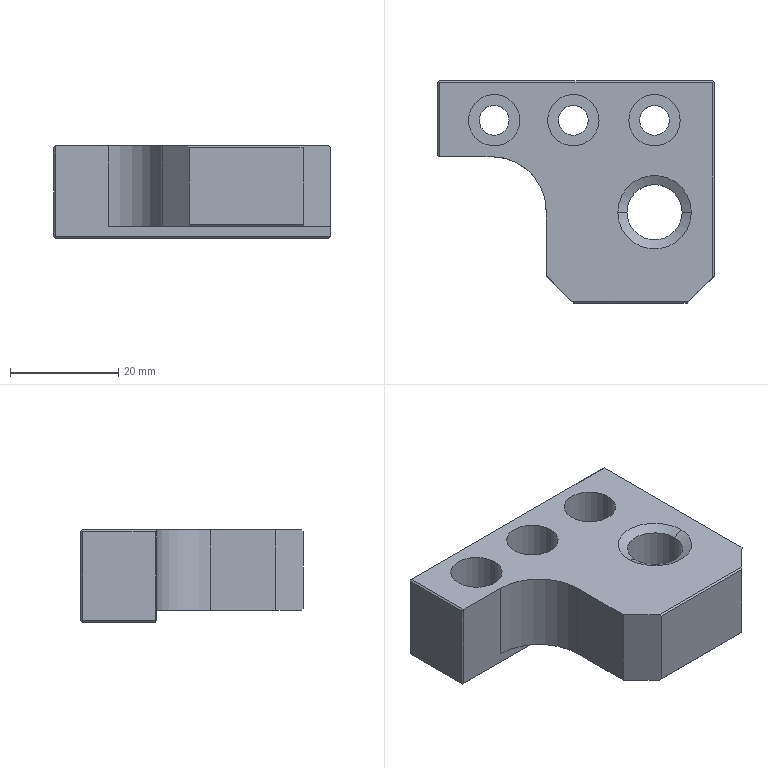Part | NX | 1 solid | 43 faces | box 51 x 41 x 17 mm | volume 20948 mm3 | plane 26 | cylinder 15 | cone 2 | commonest cylinder face diameters 5.5 x6 9.5 x6 10.2 x2 20 x1
STEP:
#1=CARTESIAN_POINT('',(1547.5,164.7,-33.6));
#2=VERTEX_POINT('',#1);
#3=CARTESIAN_POINT('',(1547.5,151.,-33.6));
#4=VERTEX_POINT('',#3);
#5=CARTESIAN_POINT('',(1547.5,165.,-33.6));
#6=DIRECTION('',(0.,-1.,0.));
#7=VECTOR('',#6,1000.);
#8=LINE('',#5,#7);
#9=EDGE_CURVE('',#2,#4,#8,.T.);
#10=ORIENTED_EDGE('',*,*,#9,.F.);
#11=CARTESIAN_POINT('',(1547.5,164.7,-17.2));
#12=VERTEX_POINT('',#11);
#13=CARTESIAN_POINT('',(1547.5,164.7,-25.4));
#14=DIRECTION('',(0.,0.,-1.));
#15=VECTOR('',#14,1000.);
#16=LINE('',#13,#15);
#17=EDGE_CURVE('',#12,#2,#16,.T.);
#18=ORIENTED_EDGE('',*,*,#17,.F.);
#19=CARTESIAN_POINT('',(1547.5,129.,-17.2));
#20=VERTEX_POINT('',#19);
#21=CARTESIAN_POINT('',(1547.5,147.,-17.2));
#22=DIRECTION('',(0.,-1.,0.));
#23=VECTOR('',#22,1000.);
#24=LINE('',#21,#23);
#25=EDGE_CURVE('',#12,#20,#24,.T.);
#26=ORIENTED_EDGE('',*,*,#25,.T.);
#27=CARTESIAN_POINT('',(1547.5,129.,-31.7));
#28=VERTEX_POINT('',#27);
#29=CARTESIAN_POINT('',(1547.5,129.,-24.3));
#30=DIRECTION('',(0.,0.,1.));
#31=VECTOR('',#30,1000.);
#32=LINE('',#29,#31);
#33=EDGE_CURVE('',#28,#20,#32,.T.);
#34=ORIENTED_EDGE('',*,*,#33,.F.);
#35=CARTESIAN_POINT('',(1547.5,151.,-31.7));
#36=VERTEX_POINT('',#35);
#37=CARTESIAN_POINT('',(1547.5,165.,-31.7));
#38=DIRECTION('',(0.,-1.,0.));
#39=VECTOR('',#38,1000.);
#40=LINE('',#37,#39);
#41=EDGE_CURVE('',#36,#28,#40,.T.);
#42=ORIENTED_EDGE('',*,*,#41,.F.);
#43=CARTESIAN_POINT('',(1547.5,151.,-40.046));
#44=DIRECTION('',(0.,0.,1.));
#45=VECTOR('',#44,1000.);
#46=LINE('',#43,#45);
#47=EDGE_CURVE('',#4,#36,#46,.T.);
#48=ORIENTED_EDGE('',*,*,#47,.F.);
#49=EDGE_LOOP('',(#10,#18,#26,#34,#42,#48));
#50=FACE_BOUND('',#49,.T.);
#51=CARTESIAN_POINT('',(1547.5,165.,-12.9));
#52=DIRECTION('',(1.,0.,0.));
#53=DIRECTION('',(0.,1.,0.));
#54=AXIS2_PLACEMENT_3D('',#51,#52,#53);
#55=PLANE('',#54);
#56=ADVANCED_FACE('',(#50),#55,.T.);
#57=CARTESIAN_POINT('',(1496.8,151.,-16.9));
#58=VERTEX_POINT('',#57);
#59=CARTESIAN_POINT('',(1496.8,164.7,-16.9));
#60=VERTEX_POINT('',#59);
#61=CARTESIAN_POINT('',(1496.8,165.,-16.9));
#62=DIRECTION('',(0.,1.,0.));
#63=VECTOR('',#62,1000.);
#64=LINE('',#61,#63);
#65=EDGE_CURVE('',#58,#60,#64,.T.);
#66=ORIENTED_EDGE('',*,*,#65,.F.);
#67=CARTESIAN_POINT('',(1506.5,151.,-16.9));
#68=VERTEX_POINT('',#67);
#69=CARTESIAN_POINT('',(1509.731,151.,-16.9));
#70=DIRECTION('',(-1.,0.,0.));
#71=VECTOR('',#70,1000.);
#72=LINE('',#69,#71);
#73=EDGE_CURVE('',#68,#58,#72,.T.);
#74=ORIENTED_EDGE('',*,*,#73,.F.);
#75=CARTESIAN_POINT('',(1516.5,141.,-16.9));
#76=VERTEX_POINT('',#75);
#77=CARTESIAN_POINT('',(1506.5,141.,-16.9));
#78=DIRECTION('',(0.,0.,1.));
#79=DIRECTION('',(0.,-1.,0.));
#80=AXIS2_PLACEMENT_3D('',#77,#78,#79);
#81=CIRCLE('',#80,10.);
#82=EDGE_CURVE('',#76,#68,#81,.T.);
#83=ORIENTED_EDGE('',*,*,#82,.F.);
#84=CARTESIAN_POINT('',(1516.5,129.,-16.9));
#85=VERTEX_POINT('',#84);
#86=CARTESIAN_POINT('',(1516.5,165.,-16.9));
#87=DIRECTION('',(0.,1.,0.));
#88=VECTOR('',#87,1000.);
#89=LINE('',#86,#88);
#90=EDGE_CURVE('',#85,#76,#89,.T.);
#91=ORIENTED_EDGE('',*,*,#90,.F.);
#92=CARTESIAN_POINT('',(1521.2,124.3,-16.9));
#93=VERTEX_POINT('',#92);
#94=CARTESIAN_POINT('',(1480.5,165.,-16.9));
#95=DIRECTION('',(0.7071,-0.7071,0.));
#96=VECTOR('',#95,1000.);
#97=LINE('',#94,#96);
#98=EDGE_CURVE('',#85,#93,#97,.T.);
#99=ORIENTED_EDGE('',*,*,#98,.T.);
#100=CARTESIAN_POINT('',(1542.8,124.3,-16.9));
#101=VERTEX_POINT('',#100);
#102=CARTESIAN_POINT('',(1532.,124.3,-16.9));
#103=DIRECTION('',(-1.,0.,0.));
#104=VECTOR('',#103,1000.);
#105=LINE('',#102,#104);
#106=EDGE_CURVE('',#101,#93,#105,.T.);
#107=ORIENTED_EDGE('',*,*,#106,.F.);
#108=CARTESIAN_POINT('',(1547.2,128.7,-16.9));
#109=VERTEX_POINT('',#108);
#110=CARTESIAN_POINT('',(1583.5,165.,-16.9));
#111=DIRECTION('',(-0.7071,-0.7071,0.));
#112=VECTOR('',#111,1000.);
#113=LINE('',#110,#112);
#114=EDGE_CURVE('',#109,#101,#113,.T.);
#115=ORIENTED_EDGE('',*,*,#114,.F.);
#116=CARTESIAN_POINT('',(1547.2,164.7,-16.9));
#117=VERTEX_POINT('',#116);
#118=CARTESIAN_POINT('',(1547.2,147.,-16.9));
#119=DIRECTION('',(0.,-1.,0.));
#120=VECTOR('',#119,1000.);
#121=LINE('',#118,#120);
#122=EDGE_CURVE('',#117,#109,#121,.T.);
#123=ORIENTED_EDGE('',*,*,#122,.F.);
#124=CARTESIAN_POINT('',(1522.,164.7,-16.9));
#125=DIRECTION('',(1.,0.,0.));
#126=VECTOR('',#125,1000.);
#127=LINE('',#124,#126);
#128=EDGE_CURVE('',#60,#117,#127,.T.);
#129=ORIENTED_EDGE('',*,*,#128,.F.);
#130=EDGE_LOOP('',(#66,#74,#83,#91,#99,#107,#115,#123,#129));
#131=FACE_BOUND('',#130,.T.);
#132=CARTESIAN_POINT('',(1543.287,140.75,-16.9));
#133=VERTEX_POINT('',#132);
#134=CARTESIAN_POINT('',(1529.713,140.75,-16.9));
#135=VERTEX_POINT('',#134);
#136=CARTESIAN_POINT('',(1536.5,140.75,-16.9));
#137=DIRECTION('',(0.,0.,1.));
#138=DIRECTION('',(-1.,0.,0.));
#139=AXIS2_PLACEMENT_3D('',#136,#137,#138);
#140=CIRCLE('',#139,6.787);
#141=EDGE_CURVE('',#133,#135,#140,.T.);
#142=ORIENTED_EDGE('',*,*,#141,.F.);
#143=CARTESIAN_POINT('',(1536.5,140.75,-16.9));
#144=DIRECTION('',(0.,0.,1.));
#145=DIRECTION('',(-1.,0.,0.));
#146=AXIS2_PLACEMENT_3D('',#143,#144,#145);
#147=CIRCLE('',#146,6.787);
#148=EDGE_CURVE('',#135,#133,#147,.T.);
#149=ORIENTED_EDGE('',*,*,#148,.F.);
#150=EDGE_LOOP('',(#142,#149));
#151=FACE_BOUND('',#150,.T.);
#152=CARTESIAN_POINT('',(1541.25,157.75,-16.9));
#153=VERTEX_POINT('',#152);
#154=CARTESIAN_POINT('',(1531.75,157.75,-16.9));
#155=VERTEX_POINT('',#154);
#156=CARTESIAN_POINT('',(1536.5,157.75,-16.9));
#157=DIRECTION('',(0.,0.,1.));
#158=DIRECTION('',(-1.,0.,0.));
#159=AXIS2_PLACEMENT_3D('',#156,#157,#158);
#160=CIRCLE('',#159,4.75);
#161=EDGE_CURVE('',#153,#155,#160,.T.);
#162=ORIENTED_EDGE('',*,*,#161,.F.);
#163=CARTESIAN_POINT('',(1536.5,157.75,-16.9));
#164=DIRECTION('',(0.,0.,1.));
#165=DIRECTION('',(-1.,0.,0.));
#166=AXIS2_PLACEMENT_3D('',#163,#164,#165);
#167=CIRCLE('',#166,4.75);
#168=EDGE_CURVE('',#155,#153,#167,.T.);
#169=ORIENTED_EDGE('',*,*,#168,.F.);
#170=EDGE_LOOP('',(#162,#169));
#171=FACE_BOUND('',#170,.T.);
#172=CARTESIAN_POINT('',(1511.642,157.75,-16.9));
#173=VERTEX_POINT('',#172);
#174=CARTESIAN_POINT('',(1502.142,157.75,-16.9));
#175=VERTEX_POINT('',#174);
#176=CARTESIAN_POINT('',(1506.892,157.75,-16.9));
#177=DIRECTION('',(0.,0.,1.));
#178=DIRECTION('',(-1.,0.,0.));
#179=AXIS2_PLACEMENT_3D('',#176,#177,#178);
#180=CIRCLE('',#179,4.75);
#181=EDGE_CURVE('',#173,#175,#180,.T.);
#182=ORIENTED_EDGE('',*,*,#181,.F.);
#183=CARTESIAN_POINT('',(1506.892,157.75,-16.9));
#184=DIRECTION('',(0.,0.,1.));
#185=DIRECTION('',(-1.,0.,0.));
#186=AXIS2_PLACEMENT_3D('',#183,#184,#185);
#187=CIRCLE('',#186,4.75);
#188=EDGE_CURVE('',#175,#173,#187,.T.);
#189=ORIENTED_EDGE('',*,*,#188,.F.);
#190=EDGE_LOOP('',(#182,#189));
#191=FACE_BOUND('',#190,.T.);
#192=CARTESIAN_POINT('',(1526.25,157.75,-16.9));
#193=VERTEX_POINT('',#192);
#194=CARTESIAN_POINT('',(1516.75,157.75,-16.9));
#195=VERTEX_POINT('',#194);
#196=CARTESIAN_POINT('',(1521.5,157.75,-16.9));
#197=DIRECTION('',(0.,0.,1.));
#198=DIRECTION('',(-1.,0.,0.));
#199=AXIS2_PLACEMENT_3D('',#196,#197,#198);
#200=CIRCLE('',#199,4.75);
#201=EDGE_CURVE('',#193,#195,#200,.T.);
#202=ORIENTED_EDGE('',*,*,#201,.F.);
#203=CARTESIAN_POINT('',(1521.5,157.75,-16.9));
#204=DIRECTION('',(0.,0.,1.));
#205=DIRECTION('',(-1.,0.,0.));
#206=AXIS2_PLACEMENT_3D('',#203,#204,#205);
#207=CIRCLE('',#206,4.75);
#208=EDGE_CURVE('',#195,#193,#207,.T.);
#209=ORIENTED_EDGE('',*,*,#208,.F.);
#210=EDGE_LOOP('',(#202,#209));
#211=FACE_BOUND('',#210,.T.);
#212=CARTESIAN_POINT('',(1491.5,165.,-16.9));
#213=DIRECTION('',(0.,0.,1.));
#214=DIRECTION('',(0.,-1.,0.));
#215=AXIS2_PLACEMENT_3D('',#212,#213,#214);
#216=PLANE('',#215);
#217=ADVANCED_FACE('',(#131,#151,#171,#191,#211),#216,.T.);
#218=CARTESIAN_POINT('',(1496.5,151.3,-17.2));
#219=VERTEX_POINT('',#218);
#220=CARTESIAN_POINT('',(1496.5,151.3,-33.6));
#221=VERTEX_POINT('',#220);
#222=CARTESIAN_POINT('',(1496.5,151.3,-25.4));
#223=DIRECTION('',(0.,0.,-1.));
#224=VECTOR('',#223,1000.);
#225=LINE('',#222,#224);
#226=EDGE_CURVE('',#219,#221,#225,.T.);
#227=ORIENTED_EDGE('',*,*,#226,.F.);
#228=CARTESIAN_POINT('',(1496.5,164.7,-17.2));
#229=VERTEX_POINT('',#228);
#230=CARTESIAN_POINT('',(1496.5,165.,-17.2));
#231=DIRECTION('',(0.,1.,0.));
#232=VECTOR('',#231,1000.);
#233=LINE('',#230,#232);
#234=EDGE_CURVE('',#219,#229,#233,.T.);
#235=ORIENTED_EDGE('',*,*,#234,.T.);
#236=CARTESIAN_POINT('',(1496.5,164.7,-33.6));
#237=VERTEX_POINT('',#236);
#238=CARTESIAN_POINT('',(1496.5,164.7,-25.4));
#239=DIRECTION('',(0.,0.,1.));
#240=VECTOR('',#239,1000.);
#241=LINE('',#238,#240);
#242=EDGE_CURVE('',#237,#229,#241,.T.);
#243=ORIENTED_EDGE('',*,*,#242,.F.);
#244=CARTESIAN_POINT('',(1496.5,165.,-33.6));
#245=DIRECTION('',(0.,1.,0.));
#246=VECTOR('',#245,1000.);
#247=LINE('',#244,#246);
#248=EDGE_CURVE('',#221,#237,#247,.T.);
#249=ORIENTED_EDGE('',*,*,#248,.F.);
#250=EDGE_LOOP('',(#227,#235,#243,#249));
#251=FACE_BOUND('',#250,.T.);
#252=CARTESIAN_POINT('',(1496.5,165.,-33.9));
#253=DIRECTION('',(-1.,0.,0.));
#254=DIRECTION('',(0.,0.,1.));
#255=AXIS2_PLACEMENT_3D('',#252,#253,#254);
#256=PLANE('',#255);
#257=ADVANCED_FACE('',(#251),#256,.T.);
#258=CARTESIAN_POINT('',(1496.8,151.3,-33.9));
#259=VERTEX_POINT('',#258);
#260=CARTESIAN_POINT('',(1496.8,164.7,-33.9));
#261=VERTEX_POINT('',#260);
#262=CARTESIAN_POINT('',(1496.8,165.,-33.9));
#263=DIRECTION('',(0.,1.,0.));
#264=VECTOR('',#263,1000.);
#265=LINE('',#262,#264);
#266=EDGE_CURVE('',#259,#261,#265,.T.);
#267=ORIENTED_EDGE('',*,*,#266,.T.);
#268=CARTESIAN_POINT('',(1547.2,164.7,-33.9));
#269=VERTEX_POINT('',#268);
#270=CARTESIAN_POINT('',(1522.,164.7,-33.9));
#271=DIRECTION('',(1.,0.,0.));
#272=VECTOR('',#271,1000.);
#273=LINE('',#270,#272);
#274=EDGE_CURVE('',#261,#269,#273,.T.);
#275=ORIENTED_EDGE('',*,*,#274,.T.);
#276=CARTESIAN_POINT('',(1547.2,151.3,-33.9));
#277=VERTEX_POINT('',#276);
#278=CARTESIAN_POINT('',(1547.2,165.,-33.9));
#279=DIRECTION('',(0.,-1.,0.));
#280=VECTOR('',#279,1000.);
#281=LINE('',#278,#280);
#282=EDGE_CURVE('',#269,#277,#281,.T.);
#283=ORIENTED_EDGE('',*,*,#282,.T.);
#284=CARTESIAN_POINT('',(1522.,151.3,-33.9));
#285=DIRECTION('',(1.,0.,0.));
#286=VECTOR('',#285,1000.);
#287=LINE('',#284,#286);
#288=EDGE_CURVE('',#259,#277,#287,.T.);
#289=ORIENTED_EDGE('',*,*,#288,.F.);
#290=EDGE_LOOP('',(#267,#275,#283,#289));
#291=FACE_BOUND('',#290,.T.);
#292=CARTESIAN_POINT('',(1509.642,157.75,-33.9));
#293=VERTEX_POINT('',#292);
#294=CARTESIAN_POINT('',(1504.142,157.75,-33.9));
#295=VERTEX_POINT('',#294);
#296=CARTESIAN_POINT('',(1506.892,157.75,-33.9));
#297=DIRECTION('',(0.,0.,1.));
#298=DIRECTION('',(-1.,0.,0.));
#299=AXIS2_PLACEMENT_3D('',#296,#297,#298);
#300=CIRCLE('',#299,2.75);
#301=EDGE_CURVE('',#293,#295,#300,.T.);
#302=ORIENTED_EDGE('',*,*,#301,.T.);
#303=CARTESIAN_POINT('',(1506.892,157.75,-33.9));
#304=DIRECTION('',(0.,0.,1.));
#305=DIRECTION('',(-1.,0.,0.));
#306=AXIS2_PLACEMENT_3D('',#303,#304,#305);
#307=CIRCLE('',#306,2.75);
#308=EDGE_CURVE('',#295,#293,#307,.T.);
#309=ORIENTED_EDGE('',*,*,#308,.T.);
#310=EDGE_LOOP('',(#302,#309));
#311=FACE_BOUND('',#310,.T.);
#312=CARTESIAN_POINT('',(1524.25,157.75,-33.9));
#313=VERTEX_POINT('',#312);
#314=CARTESIAN_POINT('',(1518.75,157.75,-33.9));
#315=VERTEX_POINT('',#314);
#316=CARTESIAN_POINT('',(1521.5,157.75,-33.9));
#317=DIRECTION('',(0.,0.,1.));
#318=DIRECTION('',(-1.,0.,0.));
#319=AXIS2_PLACEMENT_3D('',#316,#317,#318);
#320=CIRCLE('',#319,2.75);
#321=EDGE_CURVE('',#313,#315,#320,.T.);
#322=ORIENTED_EDGE('',*,*,#321,.T.);
#323=CARTESIAN_POINT('',(1521.5,157.75,-33.9));
#324=DIRECTION('',(0.,0.,1.));
#325=DIRECTION('',(-1.,0.,0.));
#326=AXIS2_PLACEMENT_3D('',#323,#324,#325);
#327=CIRCLE('',#326,2.75);
#328=EDGE_CURVE('',#315,#313,#327,.T.);
#329=ORIENTED_EDGE('',*,*,#328,.T.);
#330=EDGE_LOOP('',(#322,#329));
#331=FACE_BOUND('',#330,.T.);
#332=CARTESIAN_POINT('',(1539.25,157.75,-33.9));
#333=VERTEX_POINT('',#332);
#334=CARTESIAN_POINT('',(1533.75,157.75,-33.9));
#335=VERTEX_POINT('',#334);
#336=CARTESIAN_POINT('',(1536.5,157.75,-33.9));
#337=DIRECTION('',(0.,0.,1.));
#338=DIRECTION('',(-1.,0.,0.));
#339=AXIS2_PLACEMENT_3D('',#336,#337,#338);
#340=CIRCLE('',#339,2.75);
#341=EDGE_CURVE('',#333,#335,#340,.T.);
#342=ORIENTED_EDGE('',*,*,#341,.T.);
#343=CARTESIAN_POINT('',(1536.5,157.75,-33.9));
#344=DIRECTION('',(0.,0.,1.));
#345=DIRECTION('',(-1.,0.,0.));
#346=AXIS2_PLACEMENT_3D('',#343,#344,#345);
#347=CIRCLE('',#346,2.75);
#348=EDGE_CURVE('',#335,#333,#347,.T.);
#349=ORIENTED_EDGE('',*,*,#348,.T.);
#350=EDGE_LOOP('',(#342,#349));
#351=FACE_BOUND('',#350,.T.);
#352=CARTESIAN_POINT('',(1551.5,165.,-33.9));
#353=DIRECTION('',(0.,0.,-1.));
#354=DIRECTION('',(0.,-1.,0.));
#355=AXIS2_PLACEMENT_3D('',#352,#353,#354);
#356=PLANE('',#355);
#357=ADVANCED_FACE('',(#291,#311,#331,#351),#356,.T.);
#358=CARTESIAN_POINT('',(1542.8,124.3,-31.7));
#359=VERTEX_POINT('',#358);
#360=CARTESIAN_POINT('',(1521.2,124.3,-31.7));
#361=VERTEX_POINT('',#360);
#362=CARTESIAN_POINT('',(1532.,124.3,-31.7));
#363=DIRECTION('',(-1.,0.,0.));
#364=VECTOR('',#363,1000.);
#365=LINE('',#362,#364);
#366=EDGE_CURVE('',#359,#361,#365,.T.);
#367=ORIENTED_EDGE('',*,*,#366,.T.);
#368=CARTESIAN_POINT('',(1516.5,129.,-31.7));
#369=VERTEX_POINT('',#368);
#370=CARTESIAN_POINT('',(1480.5,165.,-31.7));
#371=DIRECTION('',(0.7071,-0.7071,0.));
#372=VECTOR('',#371,1000.);
#373=LINE('',#370,#372);
#374=EDGE_CURVE('',#369,#361,#373,.T.);
#375=ORIENTED_EDGE('',*,*,#374,.F.);
#376=CARTESIAN_POINT('',(1516.5,141.,-31.7));
#377=VERTEX_POINT('',#376);
#378=CARTESIAN_POINT('',(1516.5,165.,-31.7));
#379=DIRECTION('',(0.,1.,0.));
#380=VECTOR('',#379,1000.);
#381=LINE('',#378,#380);
#382=EDGE_CURVE('',#369,#377,#381,.T.);
#383=ORIENTED_EDGE('',*,*,#382,.T.);
#384=CARTESIAN_POINT('',(1506.5,151.,-31.7));
#385=VERTEX_POINT('',#384);
#386=CARTESIAN_POINT('',(1506.5,141.,-31.7));
#387=DIRECTION('',(0.,0.,1.));
#388=DIRECTION('',(0.,-1.,0.));
#389=AXIS2_PLACEMENT_3D('',#386,#387,#388);
#390=CIRCLE('',#389,10.);
#391=EDGE_CURVE('',#377,#385,#390,.T.);
#392=ORIENTED_EDGE('',*,*,#391,.T.);
#393=CARTESIAN_POINT('',(1509.731,151.,-31.7));
#394=DIRECTION('',(-1.,0.,0.));
#395=VECTOR('',#394,1000.);
#396=LINE('',#393,#395);
#397=EDGE_CURVE('',#36,#385,#396,.T.);
#398=ORIENTED_EDGE('',*,*,#397,.F.);
#399=ORIENTED_EDGE('',*,*,#41,.T.);
#400=CARTESIAN_POINT('',(1583.5,165.,-31.7));
#401=DIRECTION('',(-0.7071,-0.7071,0.));
#402=VECTOR('',#401,1000.);
#403=LINE('',#400,#402);
#404=EDGE_CURVE('',#28,#359,#403,.T.);
#405=ORIENTED_EDGE('',*,*,#404,.T.);
#406=EDGE_LOOP('',(#367,#375,#383,#392,#398,#399,#405));
#407=FACE_BOUND('',#406,.T.);
#408=CARTESIAN_POINT('',(1541.6,140.75,-31.7));
#409=VERTEX_POINT('',#408);
#410=CARTESIAN_POINT('',(1531.4,140.75,-31.7));
#411=VERTEX_POINT('',#410);
#412=CARTESIAN_POINT('',(1536.5,140.75,-31.7));
#413=DIRECTION('',(0.,0.,1.));
#414=DIRECTION('',(-1.,0.,0.));
#415=AXIS2_PLACEMENT_3D('',#412,#413,#414);
#416=CIRCLE('',#415,5.1);
#417=EDGE_CURVE('',#409,#411,#416,.T.);
#418=ORIENTED_EDGE('',*,*,#417,.T.);
#419=CARTESIAN_POINT('',(1536.5,140.75,-31.7));
#420=DIRECTION('',(0.,0.,1.));
#421=DIRECTION('',(-1.,0.,0.));
#422=AXIS2_PLACEMENT_3D('',#419,#420,#421);
#423=CIRCLE('',#422,5.1);
#424=EDGE_CURVE('',#411,#409,#423,.T.);
#425=ORIENTED_EDGE('',*,*,#424,.T.);
#426=EDGE_LOOP('',(#418,#425));
#427=FACE_BOUND('',#426,.T.);
#428=CARTESIAN_POINT('',(1491.4,105.,-31.7));
#429=DIRECTION('',(0.,0.,1.));
#430=DIRECTION('',(1.,0.,0.));
#431=AXIS2_PLACEMENT_3D('',#428,#429,#430);
#432=PLANE('',#431);
#433=ADVANCED_FACE('',(#407,#427),#432,.F.);
#434=CARTESIAN_POINT('',(1496.8,151.,-33.6));
#435=VERTEX_POINT('',#434);
#436=CARTESIAN_POINT('',(1522.,151.,-33.6));
#437=DIRECTION('',(1.,0.,0.));
#438=VECTOR('',#437,1000.);
#439=LINE('',#436,#438);
#440=EDGE_CURVE('',#435,#4,#439,.T.);
#441=ORIENTED_EDGE('',*,*,#440,.T.);
#442=ORIENTED_EDGE('',*,*,#47,.T.);
#443=ORIENTED_EDGE('',*,*,#397,.T.);
#444=CARTESIAN_POINT('',(1506.5,151.,-40.046));
#445=DIRECTION('',(0.,0.,1.));
#446=VECTOR('',#445,1000.);
#447=LINE('',#444,#446);
#448=EDGE_CURVE('',#385,#68,#447,.T.);
#449=ORIENTED_EDGE('',*,*,#448,.T.);
#450=ORIENTED_EDGE('',*,*,#73,.T.);
#451=CARTESIAN_POINT('',(1496.8,151.,-25.4));
#452=DIRECTION('',(0.,0.,-1.));
#453=VECTOR('',#452,1000.);
#454=LINE('',#451,#453);
#455=EDGE_CURVE('',#58,#435,#454,.T.);
#456=ORIENTED_EDGE('',*,*,#455,.T.);
#457=EDGE_LOOP('',(#441,#442,#443,#449,#450,#456));
#458=FACE_BOUND('',#457,.T.);
#459=CARTESIAN_POINT('',(1491.4,151.,-31.7));
#460=DIRECTION('',(0.,1.,0.));
#461=DIRECTION('',(1.,0.,0.));
#462=AXIS2_PLACEMENT_3D('',#459,#460,#461);
#463=PLANE('',#462);
#464=ADVANCED_FACE('',(#458),#463,.F.);
#465=CARTESIAN_POINT('',(1509.642,157.75,-24.4));
#466=VERTEX_POINT('',#465);
#467=CARTESIAN_POINT('',(1504.142,157.75,-24.4));
#468=VERTEX_POINT('',#467);
#469=CARTESIAN_POINT('',(1506.892,157.75,-24.4));
#470=DIRECTION('',(0.,0.,1.));
#471=DIRECTION('',(-1.,0.,0.));
#472=AXIS2_PLACEMENT_3D('',#469,#470,#471);
#473=CIRCLE('',#472,2.75);
#474=EDGE_CURVE('',#466,#468,#473,.T.);
#475=ORIENTED_EDGE('',*,*,#474,.T.);
#476=CARTESIAN_POINT('',(1504.142,157.75,-16.9));
#477=DIRECTION('',(0.,0.,1.));
#478=VECTOR('',#477,1000.);
#479=LINE('',#476,#478);
#480=EDGE_CURVE('',#295,#468,#479,.T.);
#481=ORIENTED_EDGE('',*,*,#480,.F.);
#482=ORIENTED_EDGE('',*,*,#301,.F.);
#483=CARTESIAN_POINT('',(1509.642,157.75,-16.9));
#484=DIRECTION('',(0.,0.,1.));
#485=VECTOR('',#484,1000.);
#486=LINE('',#483,#485);
#487=EDGE_CURVE('',#293,#466,#486,.T.);
#488=ORIENTED_EDGE('',*,*,#487,.T.);
#489=EDGE_LOOP('',(#475,#481,#482,#488));
#490=FACE_BOUND('',#489,.T.);
#491=CARTESIAN_POINT('',(1506.892,157.75,-16.9));
#492=DIRECTION('',(0.,0.,1.));
#493=DIRECTION('',(-1.,0.,0.));
#494=AXIS2_PLACEMENT_3D('',#491,#492,#493);
#495=CYLINDRICAL_SURFACE('',#494,2.75);
#496=ADVANCED_FACE('',(#490),#495,.F.);
#497=CARTESIAN_POINT('',(1511.642,157.75,-24.4));
#498=VERTEX_POINT('',#497);
#499=CARTESIAN_POINT('',(1502.142,157.75,-24.4));
#500=VERTEX_POINT('',#499);
#501=CARTESIAN_POINT('',(1506.892,157.75,-24.4));
#502=DIRECTION('',(0.,0.,1.));
#503=DIRECTION('',(-1.,0.,0.));
#504=AXIS2_PLACEMENT_3D('',#501,#502,#503);
#505=CIRCLE('',#504,4.75);
#506=EDGE_CURVE('',#498,#500,#505,.T.);
#507=ORIENTED_EDGE('',*,*,#506,.T.);
#508=CARTESIAN_POINT('',(1506.892,157.75,-24.4));
#509=DIRECTION('',(0.,0.,1.));
#510=DIRECTION('',(-1.,0.,0.));
#511=AXIS2_PLACEMENT_3D('',#508,#509,#510);
#512=CIRCLE('',#511,4.75);
#513=EDGE_CURVE('',#500,#498,#512,.T.);
#514=ORIENTED_EDGE('',*,*,#513,.T.);
#515=EDGE_LOOP('',(#507,#514));
#516=FACE_BOUND('',#515,.T.);
#517=ORIENTED_EDGE('',*,*,#474,.F.);
#518=CARTESIAN_POINT('',(1506.892,157.75,-24.4));
#519=DIRECTION('',(0.,0.,1.));
#520=DIRECTION('',(-1.,0.,0.));
#521=AXIS2_PLACEMENT_3D('',#518,#519,#520);
#522=CIRCLE('',#521,2.75);
#523=EDGE_CURVE('',#468,#466,#522,.T.);
#524=ORIENTED_EDGE('',*,*,#523,.F.);
#525=EDGE_LOOP('',(#517,#524));
#526=FACE_BOUND('',#525,.T.);
#527=CARTESIAN_POINT('',(1506.892,157.75,-24.4));
#528=DIRECTION('',(0.,0.,1.));
#529=DIRECTION('',(0.,-1.,0.));
#530=AXIS2_PLACEMENT_3D('',#527,#528,#529);
#531=PLANE('',#530);
#532=ADVANCED_FACE('',(#516,#526),#531,.T.);
#533=ORIENTED_EDGE('',*,*,#181,.T.);
#534=CARTESIAN_POINT('',(1502.142,157.75,-16.9));
#535=DIRECTION('',(0.,0.,1.));
#536=VECTOR('',#535,1000.);
#537=LINE('',#534,#536);
#538=EDGE_CURVE('',#175,#500,#537,.F.);
#539=ORIENTED_EDGE('',*,*,#538,.T.);
#540=ORIENTED_EDGE('',*,*,#506,.F.);
#541=CARTESIAN_POINT('',(1511.642,157.75,-16.9));
#542=DIRECTION('',(0.,0.,1.));
#543=VECTOR('',#542,1000.);
#544=LINE('',#541,#543);
#545=EDGE_CURVE('',#173,#498,#544,.F.);
#546=ORIENTED_EDGE('',*,*,#545,.F.);
#547=EDGE_LOOP('',(#533,#539,#540,#546));
#548=FACE_BOUND('',#547,.T.);
#549=CARTESIAN_POINT('',(1506.892,157.75,-16.9));
#550=DIRECTION('',(0.,0.,1.));
#551=DIRECTION('',(-1.,0.,0.));
#552=AXIS2_PLACEMENT_3D('',#549,#550,#551);
#553=CYLINDRICAL_SURFACE('',#552,4.75);
#554=ADVANCED_FACE('',(#548),#553,.F.);
#555=ORIENTED_EDGE('',*,*,#201,.T.);
#556=CARTESIAN_POINT('',(1516.75,157.75,-24.4));
#557=VERTEX_POINT('',#556);
#558=CARTESIAN_POINT('',(1516.75,157.75,-16.9));
#559=DIRECTION('',(0.,0.,1.));
#560=VECTOR('',#559,1000.);
#561=LINE('',#558,#560);
#562=EDGE_CURVE('',#195,#557,#561,.F.);
#563=ORIENTED_EDGE('',*,*,#562,.T.);
#564=CARTESIAN_POINT('',(1526.25,157.75,-24.4));
#565=VERTEX_POINT('',#564);
#566=CARTESIAN_POINT('',(1521.5,157.75,-24.4));
#567=DIRECTION('',(0.,0.,1.));
#568=DIRECTION('',(-1.,0.,0.));
#569=AXIS2_PLACEMENT_3D('',#566,#567,#568);
#570=CIRCLE('',#569,4.75);
#571=EDGE_CURVE('',#565,#557,#570,.T.);
#572=ORIENTED_EDGE('',*,*,#571,.F.);
#573=CARTESIAN_POINT('',(1526.25,157.75,-16.9));
#574=DIRECTION('',(0.,0.,1.));
#575=VECTOR('',#574,1000.);
#576=LINE('',#573,#575);
#577=EDGE_CURVE('',#193,#565,#576,.F.);
#578=ORIENTED_EDGE('',*,*,#577,.F.);
#579=EDGE_LOOP('',(#555,#563,#572,#578));
#580=FACE_BOUND('',#579,.T.);
#581=CARTESIAN_POINT('',(1521.5,157.75,-16.9));
#582=DIRECTION('',(0.,0.,1.));
#583=DIRECTION('',(-1.,0.,0.));
#584=AXIS2_PLACEMENT_3D('',#581,#582,#583);
#585=CYLINDRICAL_SURFACE('',#584,4.75);
#586=ADVANCED_FACE('',(#580),#585,.F.);
#587=ORIENTED_EDGE('',*,*,#571,.T.);
#588=CARTESIAN_POINT('',(1521.5,157.75,-24.4));
#589=DIRECTION('',(0.,0.,1.));
#590=DIRECTION('',(-1.,0.,0.));
#591=AXIS2_PLACEMENT_3D('',#588,#589,#590);
#592=CIRCLE('',#591,4.75);
#593=EDGE_CURVE('',#557,#565,#592,.T.);
#594=ORIENTED_EDGE('',*,*,#593,.T.);
#595=EDGE_LOOP('',(#587,#594));
#596=FACE_BOUND('',#595,.T.);
#597=CARTESIAN_POINT('',(1524.25,157.75,-24.4));
#598=VERTEX_POINT('',#597);
#599=CARTESIAN_POINT('',(1518.75,157.75,-24.4));
#600=VERTEX_POINT('',#599);
#601=CARTESIAN_POINT('',(1521.5,157.75,-24.4));
#602=DIRECTION('',(0.,0.,1.));
#603=DIRECTION('',(-1.,0.,0.));
#604=AXIS2_PLACEMENT_3D('',#601,#602,#603);
#605=CIRCLE('',#604,2.75);
#606=EDGE_CURVE('',#598,#600,#605,.T.);
#607=ORIENTED_EDGE('',*,*,#606,.F.);
#608=CARTESIAN_POINT('',(1521.5,157.75,-24.4));
#609=DIRECTION('',(0.,0.,1.));
#610=DIRECTION('',(-1.,0.,0.));
#611=AXIS2_PLACEMENT_3D('',#608,#609,#610);
#612=CIRCLE('',#611,2.75);
#613=EDGE_CURVE('',#600,#598,#612,.T.);
#614=ORIENTED_EDGE('',*,*,#613,.F.);
#615=EDGE_LOOP('',(#607,#614));
#616=FACE_BOUND('',#615,.T.);
#617=CARTESIAN_POINT('',(1521.5,157.75,-24.4));
#618=DIRECTION('',(0.,0.,1.));
#619=DIRECTION('',(0.,-1.,0.));
#620=AXIS2_PLACEMENT_3D('',#617,#618,#619);
#621=PLANE('',#620);
#622=ADVANCED_FACE('',(#596,#616),#621,.T.);
#623=ORIENTED_EDGE('',*,*,#606,.T.);
#624=CARTESIAN_POINT('',(1518.75,157.75,-16.9));
#625=DIRECTION('',(0.,0.,1.));
#626=VECTOR('',#625,1000.);
#627=LINE('',#624,#626);
#628=EDGE_CURVE('',#315,#600,#627,.T.);
#629=ORIENTED_EDGE('',*,*,#628,.F.);
#630=ORIENTED_EDGE('',*,*,#321,.F.);
#631=CARTESIAN_POINT('',(1524.25,157.75,-16.9));
#632=DIRECTION('',(0.,0.,1.));
#633=VECTOR('',#632,1000.);
#634=LINE('',#631,#633);
#635=EDGE_CURVE('',#313,#598,#634,.T.);
#636=ORIENTED_EDGE('',*,*,#635,.T.);
#637=EDGE_LOOP('',(#623,#629,#630,#636));
#638=FACE_BOUND('',#637,.T.);
#639=CARTESIAN_POINT('',(1521.5,157.75,-16.9));
#640=DIRECTION('',(0.,0.,1.));
#641=DIRECTION('',(-1.,0.,0.));
#642=AXIS2_PLACEMENT_3D('',#639,#640,#641);
#643=CYLINDRICAL_SURFACE('',#642,2.75);
#644=ADVANCED_FACE('',(#638),#643,.F.);
#645=ORIENTED_EDGE('',*,*,#161,.T.);
#646=CARTESIAN_POINT('',(1531.75,157.75,-24.4));
#647=VERTEX_POINT('',#646);
#648=CARTESIAN_POINT('',(1531.75,157.75,-16.9));
#649=DIRECTION('',(0.,0.,1.));
#650=VECTOR('',#649,1000.);
#651=LINE('',#648,#650);
#652=EDGE_CURVE('',#155,#647,#651,.F.);
#653=ORIENTED_EDGE('',*,*,#652,.T.);
#654=CARTESIAN_POINT('',(1541.25,157.75,-24.4));
#655=VERTEX_POINT('',#654);
#656=CARTESIAN_POINT('',(1536.5,157.75,-24.4));
#657=DIRECTION('',(0.,0.,1.));
#658=DIRECTION('',(-1.,0.,0.));
#659=AXIS2_PLACEMENT_3D('',#656,#657,#658);
#660=CIRCLE('',#659,4.75);
#661=EDGE_CURVE('',#655,#647,#660,.T.);
#662=ORIENTED_EDGE('',*,*,#661,.F.);
#663=CARTESIAN_POINT('',(1541.25,157.75,-16.9));
#664=DIRECTION('',(0.,0.,1.));
#665=VECTOR('',#664,1000.);
#666=LINE('',#663,#665);
#667=EDGE_CURVE('',#153,#655,#666,.F.);
#668=ORIENTED_EDGE('',*,*,#667,.F.);
#669=EDGE_LOOP('',(#645,#653,#662,#668));
#670=FACE_BOUND('',#669,.T.);
#671=CARTESIAN_POINT('',(1536.5,157.75,-16.9));
#672=DIRECTION('',(0.,0.,1.));
#673=DIRECTION('',(-1.,0.,0.));
#674=AXIS2_PLACEMENT_3D('',#671,#672,#673);
#675=CYLINDRICAL_SURFACE('',#674,4.75);
#676=ADVANCED_FACE('',(#670),#675,.F.);
#677=ORIENTED_EDGE('',*,*,#661,.T.);
#678=CARTESIAN_POINT('',(1536.5,157.75,-24.4));
#679=DIRECTION('',(0.,0.,1.));
#680=DIRECTION('',(-1.,0.,0.));
#681=AXIS2_PLACEMENT_3D('',#678,#679,#680);
#682=CIRCLE('',#681,4.75);
#683=EDGE_CURVE('',#647,#655,#682,.T.);
#684=ORIENTED_EDGE('',*,*,#683,.T.);
#685=EDGE_LOOP('',(#677,#684));
#686=FACE_BOUND('',#685,.T.);
#687=CARTESIAN_POINT('',(1539.25,157.75,-24.4));
#688=VERTEX_POINT('',#687);
#689=CARTESIAN_POINT('',(1533.75,157.75,-24.4));
#690=VERTEX_POINT('',#689);
#691=CARTESIAN_POINT('',(1536.5,157.75,-24.4));
#692=DIRECTION('',(0.,0.,1.));
#693=DIRECTION('',(-1.,0.,0.));
#694=AXIS2_PLACEMENT_3D('',#691,#692,#693);
#695=CIRCLE('',#694,2.75);
#696=EDGE_CURVE('',#688,#690,#695,.T.);
#697=ORIENTED_EDGE('',*,*,#696,.F.);
#698=CARTESIAN_POINT('',(1536.5,157.75,-24.4));
#699=DIRECTION('',(0.,0.,1.));
#700=DIRECTION('',(-1.,0.,0.));
#701=AXIS2_PLACEMENT_3D('',#698,#699,#700);
#702=CIRCLE('',#701,2.75);
#703=EDGE_CURVE('',#690,#688,#702,.T.);
#704=ORIENTED_EDGE('',*,*,#703,.F.);
#705=EDGE_LOOP('',(#697,#704));
#706=FACE_BOUND('',#705,.T.);
#707=CARTESIAN_POINT('',(1536.5,157.75,-24.4));
#708=DIRECTION('',(0.,0.,1.));
#709=DIRECTION('',(0.,-1.,0.));
#710=AXIS2_PLACEMENT_3D('',#707,#708,#709);
#711=PLANE('',#710);
#712=ADVANCED_FACE('',(#686,#706),#711,.T.);
#713=ORIENTED_EDGE('',*,*,#696,.T.);
#714=CARTESIAN_POINT('',(1533.75,157.75,-16.9));
#715=DIRECTION('',(0.,0.,1.));
#716=VECTOR('',#715,1000.);
#717=LINE('',#714,#716);
#718=EDGE_CURVE('',#335,#690,#717,.T.);
#719=ORIENTED_EDGE('',*,*,#718,.F.);
#720=ORIENTED_EDGE('',*,*,#341,.F.);
#721=CARTESIAN_POINT('',(1539.25,157.75,-16.9));
#722=DIRECTION('',(0.,0.,1.));
#723=VECTOR('',#722,1000.);
#724=LINE('',#721,#723);
#725=EDGE_CURVE('',#333,#688,#724,.T.);
#726=ORIENTED_EDGE('',*,*,#725,.T.);
#727=EDGE_LOOP('',(#713,#719,#720,#726));
#728=FACE_BOUND('',#727,.T.);
#729=CARTESIAN_POINT('',(1536.5,157.75,-16.9));
#730=DIRECTION('',(0.,0.,1.));
#731=DIRECTION('',(-1.,0.,0.));
#732=AXIS2_PLACEMENT_3D('',#729,#730,#731);
#733=CYLINDRICAL_SURFACE('',#732,2.75);
#734=ADVANCED_FACE('',(#728),#733,.F.);
#735=CARTESIAN_POINT('',(1516.5,141.,-40.046));
#736=DIRECTION('',(0.,0.,1.));
#737=VECTOR('',#736,1000.);
#738=LINE('',#735,#737);
#739=EDGE_CURVE('',#377,#76,#738,.T.);
#740=ORIENTED_EDGE('',*,*,#739,.F.);
#741=ORIENTED_EDGE('',*,*,#382,.F.);
#742=CARTESIAN_POINT('',(1516.5,129.,-24.3));
#743=DIRECTION('',(0.,0.,1.));
#744=VECTOR('',#743,1000.);
#745=LINE('',#742,#744);
#746=EDGE_CURVE('',#369,#85,#745,.T.);
#747=ORIENTED_EDGE('',*,*,#746,.T.);
#748=ORIENTED_EDGE('',*,*,#90,.T.);
#749=EDGE_LOOP('',(#740,#741,#747,#748));
#750=FACE_BOUND('',#749,.T.);
#751=CARTESIAN_POINT('',(1516.5,145.,-35.6));
#752=DIRECTION('',(1.,0.,0.));
#753=DIRECTION('',(0.,1.,0.));
#754=AXIS2_PLACEMENT_3D('',#751,#752,#753);
#755=PLANE('',#754);
#756=ADVANCED_FACE('',(#750),#755,.F.);
#757=ORIENTED_EDGE('',*,*,#266,.F.);
#758=CARTESIAN_POINT('',(1496.65,151.15,-33.75));
#759=VERTEX_POINT('',#758);
#760=CARTESIAN_POINT('',(1510.5,165.,-47.6));
#761=DIRECTION('',(-0.5774,-0.5774,0.5774));
#762=VECTOR('',#761,1000.);
#763=LINE('',#760,#762);
#764=EDGE_CURVE('',#259,#759,#763,.T.);
#765=ORIENTED_EDGE('',*,*,#764,.T.);
#766=CARTESIAN_POINT('',(1502.946,144.854,-40.046));
#767=DIRECTION('',(-0.5774,0.5774,0.5774));
#768=VECTOR('',#767,1000.);
#769=LINE('',#766,#768);
#770=EDGE_CURVE('',#759,#221,#769,.T.);
#771=ORIENTED_EDGE('',*,*,#770,.T.);
#772=ORIENTED_EDGE('',*,*,#248,.T.);
#773=CARTESIAN_POINT('',(1496.65,164.85,-33.75));
#774=VERTEX_POINT('',#773);
#775=CARTESIAN_POINT('',(1502.946,171.146,-40.046));
#776=DIRECTION('',(0.5774,0.5774,-0.5774));
#777=VECTOR('',#776,1000.);
#778=LINE('',#775,#777);
#779=EDGE_CURVE('',#237,#774,#778,.T.);
#780=ORIENTED_EDGE('',*,*,#779,.T.);
#781=CARTESIAN_POINT('',(1496.5,165.,-33.6));
#782=DIRECTION('',(-0.5774,0.5774,0.5774));
#783=VECTOR('',#782,1000.);
#784=LINE('',#781,#783);
#785=EDGE_CURVE('',#261,#774,#784,.T.);
#786=ORIENTED_EDGE('',*,*,#785,.F.);
#787=EDGE_LOOP('',(#757,#765,#771,#772,#780,#786));
#788=FACE_BOUND('',#787,.T.);
#789=CARTESIAN_POINT('',(1496.65,155.5,-33.75));
#790=DIRECTION('',(0.7071,0.,0.7071));
#791=DIRECTION('',(0.,-1.,0.));
#792=AXIS2_PLACEMENT_3D('',#789,#790,#791);
#793=PLANE('',#792);
#794=ADVANCED_FACE('',(#788),#793,.F.);
#795=CARTESIAN_POINT('',(1541.6,140.75,-17.874));
#796=VERTEX_POINT('',#795);
#797=CARTESIAN_POINT('',(1531.4,140.75,-17.874));
#798=VERTEX_POINT('',#797);
#799=CARTESIAN_POINT('',(1536.5,140.75,-17.874));
#800=DIRECTION('',(0.,0.,1.));
#801=DIRECTION('',(-1.,0.,0.));
#802=AXIS2_PLACEMENT_3D('',#799,#800,#801);
#803=CIRCLE('',#802,5.1);
#804=EDGE_CURVE('',#796,#798,#803,.T.);
#805=ORIENTED_EDGE('',*,*,#804,.T.);
#806=CARTESIAN_POINT('',(1531.4,140.75,-16.9));
#807=DIRECTION('',(0.,0.,1.));
#808=VECTOR('',#807,1000.);
#809=LINE('',#806,#808);
#810=EDGE_CURVE('',#798,#411,#809,.F.);
#811=ORIENTED_EDGE('',*,*,#810,.T.);
#812=ORIENTED_EDGE('',*,*,#417,.F.);
#813=CARTESIAN_POINT('',(1541.6,140.75,-16.9));
#814=DIRECTION('',(0.,0.,1.));
#815=VECTOR('',#814,1000.);
#816=LINE('',#813,#815);
#817=EDGE_CURVE('',#796,#409,#816,.F.);
#818=ORIENTED_EDGE('',*,*,#817,.F.);
#819=EDGE_LOOP('',(#805,#811,#812,#818));
#820=FACE_BOUND('',#819,.T.);
#821=CARTESIAN_POINT('',(1536.5,140.75,-16.9));
#822=DIRECTION('',(0.,0.,1.));
#823=DIRECTION('',(-1.,0.,0.));
#824=AXIS2_PLACEMENT_3D('',#821,#822,#823);
#825=CYLINDRICAL_SURFACE('',#824,5.1);
#826=ADVANCED_FACE('',(#820),#825,.F.);
#827=ORIENTED_EDGE('',*,*,#804,.F.);
#828=CARTESIAN_POINT('',(1541.6,140.75,-17.874));
#829=DIRECTION('',(0.866,0.,0.5));
#830=VECTOR('',#829,1000.);
#831=LINE('',#828,#830);
#832=EDGE_CURVE('',#133,#796,#831,.F.);
#833=ORIENTED_EDGE('',*,*,#832,.F.);
#834=ORIENTED_EDGE('',*,*,#141,.T.);
#835=CARTESIAN_POINT('',(1531.4,140.75,-17.874));
#836=DIRECTION('',(-0.866,0.,0.5));
#837=VECTOR('',#836,1000.);
#838=LINE('',#835,#837);
#839=EDGE_CURVE('',#135,#798,#838,.F.);
#840=ORIENTED_EDGE('',*,*,#839,.T.);
#841=EDGE_LOOP('',(#827,#833,#834,#840));
#842=FACE_BOUND('',#841,.T.);
#843=CARTESIAN_POINT('',(1536.5,140.75,-17.874));
#844=DIRECTION('',(0.,0.,1.));
#845=DIRECTION('',(-1.,0.,0.));
#846=AXIS2_PLACEMENT_3D('',#843,#844,#845);
#847=CONICAL_SURFACE('',#846,5.1,1.047);
#848=ADVANCED_FACE('',(#842),#847,.F.);
#849=ORIENTED_EDGE('',*,*,#25,.F.);
#850=CARTESIAN_POINT('',(1547.35,164.85,-17.05));
#851=VERTEX_POINT('',#850);
#852=CARTESIAN_POINT('',(1570.346,141.854,-40.046));
#853=DIRECTION('',(-0.5774,0.5774,0.5774));
#854=VECTOR('',#853,1000.);
#855=LINE('',#852,#854);
#856=EDGE_CURVE('',#12,#851,#855,.T.);
#857=ORIENTED_EDGE('',*,*,#856,.T.);
#858=CARTESIAN_POINT('',(1570.346,187.846,-40.046));
#859=DIRECTION('',(0.5774,0.5774,-0.5774));
#860=VECTOR('',#859,1000.);
#861=LINE('',#858,#860);
#862=EDGE_CURVE('',#117,#851,#861,.T.);
#863=ORIENTED_EDGE('',*,*,#862,.F.);
#864=ORIENTED_EDGE('',*,*,#122,.T.);
#865=CARTESIAN_POINT('',(1570.346,151.846,-40.046));
#866=DIRECTION('',(0.5774,0.5774,-0.5774));
#867=VECTOR('',#866,1000.);
#868=LINE('',#865,#867);
#869=EDGE_CURVE('',#109,#20,#868,.T.);
#870=ORIENTED_EDGE('',*,*,#869,.T.);
#871=EDGE_LOOP('',(#849,#857,#863,#864,#870));
#872=FACE_BOUND('',#871,.T.);
#873=CARTESIAN_POINT('',(1547.35,147.,-17.05));
#874=DIRECTION('',(0.7071,0.,0.7071));
#875=DIRECTION('',(0.,-1.,0.));
#876=AXIS2_PLACEMENT_3D('',#873,#874,#875);
#877=PLANE('',#876);
#878=ADVANCED_FACE('',(#872),#877,.T.);
#879=ORIENTED_EDGE('',*,*,#366,.F.);
#880=CARTESIAN_POINT('',(1542.5,124.,-31.4));
#881=VERTEX_POINT('',#880);
#882=CARTESIAN_POINT('',(1551.146,132.646,-40.046));
#883=DIRECTION('',(-0.5774,-0.5774,0.5774));
#884=VECTOR('',#883,1000.);
#885=LINE('',#882,#884);
#886=EDGE_CURVE('',#359,#881,#885,.T.);
#887=ORIENTED_EDGE('',*,*,#886,.T.);
#888=CARTESIAN_POINT('',(1521.5,124.,-31.4));
#889=VERTEX_POINT('',#888);
#890=CARTESIAN_POINT('',(1532.,124.,-31.4));
#891=DIRECTION('',(-1.,0.,0.));
#892=VECTOR('',#891,1000.);
#893=LINE('',#890,#892);
#894=EDGE_CURVE('',#881,#889,#893,.T.);
#895=ORIENTED_EDGE('',*,*,#894,.T.);
#896=CARTESIAN_POINT('',(1512.854,132.646,-40.046));
#897=DIRECTION('',(0.5774,-0.5774,0.5774));
#898=VECTOR('',#897,1000.);
#899=LINE('',#896,#898);
#900=EDGE_CURVE('',#361,#889,#899,.T.);
#901=ORIENTED_EDGE('',*,*,#900,.F.);
#902=EDGE_LOOP('',(#879,#887,#895,#901));
#903=FACE_BOUND('',#902,.T.);
#904=CARTESIAN_POINT('',(1532.,124.15,-31.55));
#905=DIRECTION('',(0.,-0.7071,-0.7071));
#906=DIRECTION('',(0.,0.7071,-0.7071));
#907=AXIS2_PLACEMENT_3D('',#904,#905,#906);
#908=PLANE('',#907);
#909=ADVANCED_FACE('',(#903),#908,.T.);
#910=CARTESIAN_POINT('',(1482.8,165.,-30.9));
#911=DIRECTION('',(0.5774,-0.5774,0.5774));
#912=VECTOR('',#911,1000.);
#913=LINE('',#910,#912);
#914=EDGE_CURVE('',#219,#58,#913,.T.);
#915=ORIENTED_EDGE('',*,*,#914,.T.);
#916=ORIENTED_EDGE('',*,*,#65,.T.);
#917=CARTESIAN_POINT('',(1496.65,164.85,-17.05));
#918=VERTEX_POINT('',#917);
#919=CARTESIAN_POINT('',(1473.654,187.846,-40.046));
#920=DIRECTION('',(-0.5774,0.5774,-0.5774));
#921=VECTOR('',#920,1000.);
#922=LINE('',#919,#921);
#923=EDGE_CURVE('',#60,#918,#922,.T.);
#924=ORIENTED_EDGE('',*,*,#923,.T.);
#925=CARTESIAN_POINT('',(1473.654,141.854,-40.046));
#926=DIRECTION('',(0.5774,0.5774,0.5774));
#927=VECTOR('',#926,1000.);
#928=LINE('',#925,#927);
#929=EDGE_CURVE('',#229,#918,#928,.T.);
#930=ORIENTED_EDGE('',*,*,#929,.F.);
#931=ORIENTED_EDGE('',*,*,#234,.F.);
#932=EDGE_LOOP('',(#915,#916,#924,#930,#931));
#933=FACE_BOUND('',#932,.T.);
#934=CARTESIAN_POINT('',(1496.65,155.5,-17.05));
#935=DIRECTION('',(0.7071,0.,-0.7071));
#936=DIRECTION('',(0.,-1.,0.));
#937=AXIS2_PLACEMENT_3D('',#934,#935,#936);
#938=PLANE('',#937);
#939=ADVANCED_FACE('',(#933),#938,.F.);
#940=ORIENTED_EDGE('',*,*,#9,.T.);
#941=CARTESIAN_POINT('',(1533.5,165.,-47.6));
#942=DIRECTION('',(-0.5774,0.5774,-0.5774));
#943=VECTOR('',#942,1000.);
#944=LINE('',#941,#943);
#945=EDGE_CURVE('',#4,#277,#944,.T.);
#946=ORIENTED_EDGE('',*,*,#945,.T.);
#947=ORIENTED_EDGE('',*,*,#282,.F.);
#948=CARTESIAN_POINT('',(1547.35,164.85,-33.75));
#949=VERTEX_POINT('',#948);
#950=CARTESIAN_POINT('',(1547.5,165.,-33.6));
#951=DIRECTION('',(0.5774,0.5774,0.5774));
#952=VECTOR('',#951,1000.);
#953=LINE('',#950,#952);
#954=EDGE_CURVE('',#269,#949,#953,.T.);
#955=ORIENTED_EDGE('',*,*,#954,.T.);
#956=CARTESIAN_POINT('',(1541.054,171.146,-40.046));
#957=DIRECTION('',(-0.5774,0.5774,-0.5774));
#958=VECTOR('',#957,1000.);
#959=LINE('',#956,#958);
#960=EDGE_CURVE('',#2,#949,#959,.T.);
#961=ORIENTED_EDGE('',*,*,#960,.F.);
#962=EDGE_LOOP('',(#940,#946,#947,#955,#961));
#963=FACE_BOUND('',#962,.T.);
#964=CARTESIAN_POINT('',(1547.35,155.5,-33.75));
#965=DIRECTION('',(-0.7071,0.,0.7071));
#966=DIRECTION('',(0.,1.,0.));
#967=AXIS2_PLACEMENT_3D('',#964,#965,#966);
#968=PLANE('',#967);
#969=ADVANCED_FACE('',(#963),#968,.F.);
#970=ORIENTED_EDGE('',*,*,#739,.T.);
#971=ORIENTED_EDGE('',*,*,#82,.T.);
#972=ORIENTED_EDGE('',*,*,#448,.F.);
#973=ORIENTED_EDGE('',*,*,#391,.F.);
#974=EDGE_LOOP('',(#970,#971,#972,#973));
#975=FACE_BOUND('',#974,.T.);
#976=CARTESIAN_POINT('',(1506.5,141.,-40.046));
#977=DIRECTION('',(0.,0.,1.));
#978=DIRECTION('',(0.,-1.,0.));
#979=AXIS2_PLACEMENT_3D('',#976,#977,#978);
#980=CYLINDRICAL_SURFACE('',#979,10.);
#981=ADVANCED_FACE('',(#975),#980,.F.);
#982=ORIENTED_EDGE('',*,*,#455,.F.);
#983=ORIENTED_EDGE('',*,*,#914,.F.);
#984=ORIENTED_EDGE('',*,*,#226,.T.);
#985=ORIENTED_EDGE('',*,*,#770,.F.);
#986=CARTESIAN_POINT('',(1482.8,165.,-47.6));
#987=DIRECTION('',(-0.5774,0.5774,-0.5774));
#988=VECTOR('',#987,1000.);
#989=LINE('',#986,#988);
#990=EDGE_CURVE('',#435,#759,#989,.T.);
#991=ORIENTED_EDGE('',*,*,#990,.F.);
#992=EDGE_LOOP('',(#982,#983,#984,#985,#991));
#993=FACE_BOUND('',#992,.T.);
#994=CARTESIAN_POINT('',(1496.65,151.15,-25.4));
#995=DIRECTION('',(-0.7071,-0.7071,0.));
#996=DIRECTION('',(-0.7071,0.7071,0.));
#997=AXIS2_PLACEMENT_3D('',#994,#995,#996);
#998=PLANE('',#997);
#999=ADVANCED_FACE('',(#993),#998,.T.);
#1000=ORIENTED_EDGE('',*,*,#440,.F.);
#1001=ORIENTED_EDGE('',*,*,#990,.T.);
#1002=ORIENTED_EDGE('',*,*,#764,.F.);
#1003=ORIENTED_EDGE('',*,*,#288,.T.);
#1004=ORIENTED_EDGE('',*,*,#945,.F.);
#1005=EDGE_LOOP('',(#1000,#1001,#1002,#1003,#1004));
#1006=FACE_BOUND('',#1005,.T.);
#1007=CARTESIAN_POINT('',(1522.,151.15,-33.75));
#1008=DIRECTION('',(0.,-0.7071,-0.7071));
#1009=DIRECTION('',(0.,-0.7071,0.7071));
#1010=AXIS2_PLACEMENT_3D('',#1007,#1008,#1009);
#1011=PLANE('',#1010);
#1012=ADVANCED_FACE('',(#1006),#1011,.T.);
#1013=ORIENTED_EDGE('',*,*,#810,.F.);
#1014=CARTESIAN_POINT('',(1536.5,140.75,-17.874));
#1015=DIRECTION('',(0.,0.,1.));
#1016=DIRECTION('',(-1.,0.,0.));
#1017=AXIS2_PLACEMENT_3D('',#1014,#1015,#1016);
#1018=CIRCLE('',#1017,5.1);
#1019=EDGE_CURVE('',#798,#796,#1018,.T.);
#1020=ORIENTED_EDGE('',*,*,#1019,.T.);
#1021=ORIENTED_EDGE('',*,*,#817,.T.);
#1022=ORIENTED_EDGE('',*,*,#424,.F.);
#1023=EDGE_LOOP('',(#1013,#1020,#1021,#1022));
#1024=FACE_BOUND('',#1023,.T.);
#1025=CARTESIAN_POINT('',(1536.5,140.75,-16.9));
#1026=DIRECTION('',(0.,0.,1.));
#1027=DIRECTION('',(-1.,0.,0.));
#1028=AXIS2_PLACEMENT_3D('',#1025,#1026,#1027);
#1029=CYLINDRICAL_SURFACE('',#1028,5.1);
#1030=ADVANCED_FACE('',(#1024),#1029,.F.);
#1031=ORIENTED_EDGE('',*,*,#652,.F.);
#1032=ORIENTED_EDGE('',*,*,#168,.T.);
#1033=ORIENTED_EDGE('',*,*,#667,.T.);
#1034=ORIENTED_EDGE('',*,*,#683,.F.);
#1035=EDGE_LOOP('',(#1031,#1032,#1033,#1034));
#1036=FACE_BOUND('',#1035,.T.);
#1037=CARTESIAN_POINT('',(1536.5,157.75,-16.9));
#1038=DIRECTION('',(0.,0.,1.));
#1039=DIRECTION('',(-1.,0.,0.));
#1040=AXIS2_PLACEMENT_3D('',#1037,#1038,#1039);
#1041=CYLINDRICAL_SURFACE('',#1040,4.75);
#1042=ADVANCED_FACE('',(#1036),#1041,.F.);
#1043=ORIENTED_EDGE('',*,*,#562,.F.);
#1044=ORIENTED_EDGE('',*,*,#208,.T.);
#1045=ORIENTED_EDGE('',*,*,#577,.T.);
#1046=ORIENTED_EDGE('',*,*,#593,.F.);
#1047=EDGE_LOOP('',(#1043,#1044,#1045,#1046));
#1048=FACE_BOUND('',#1047,.T.);
#1049=CARTESIAN_POINT('',(1521.5,157.75,-16.9));
#1050=DIRECTION('',(0.,0.,1.));
#1051=DIRECTION('',(-1.,0.,0.));
#1052=AXIS2_PLACEMENT_3D('',#1049,#1050,#1051);
#1053=CYLINDRICAL_SURFACE('',#1052,4.75);
#1054=ADVANCED_FACE('',(#1048),#1053,.F.);
#1055=ORIENTED_EDGE('',*,*,#538,.F.);
#1056=ORIENTED_EDGE('',*,*,#188,.T.);
#1057=ORIENTED_EDGE('',*,*,#545,.T.);
#1058=ORIENTED_EDGE('',*,*,#513,.F.);
#1059=EDGE_LOOP('',(#1055,#1056,#1057,#1058));
#1060=FACE_BOUND('',#1059,.T.);
#1061=CARTESIAN_POINT('',(1506.892,157.75,-16.9));
#1062=DIRECTION('',(0.,0.,1.));
#1063=DIRECTION('',(-1.,0.,0.));
#1064=AXIS2_PLACEMENT_3D('',#1061,#1062,#1063);
#1065=CYLINDRICAL_SURFACE('',#1064,4.75);
#1066=ADVANCED_FACE('',(#1060),#1065,.F.);
#1067=ORIENTED_EDGE('',*,*,#839,.F.);
#1068=ORIENTED_EDGE('',*,*,#148,.T.);
#1069=ORIENTED_EDGE('',*,*,#832,.T.);
#1070=ORIENTED_EDGE('',*,*,#1019,.F.);
#1071=EDGE_LOOP('',(#1067,#1068,#1069,#1070));
#1072=FACE_BOUND('',#1071,.T.);
#1073=CARTESIAN_POINT('',(1536.5,140.75,-17.874));
#1074=DIRECTION('',(0.,0.,1.));
#1075=DIRECTION('',(-1.,0.,0.));
#1076=AXIS2_PLACEMENT_3D('',#1073,#1074,#1075);
#1077=CONICAL_SURFACE('',#1076,5.1,1.047);
#1078=ADVANCED_FACE('',(#1072),#1077,.F.);
#1079=ORIENTED_EDGE('',*,*,#725,.F.);
#1080=ORIENTED_EDGE('',*,*,#348,.F.);
#1081=ORIENTED_EDGE('',*,*,#718,.T.);
#1082=ORIENTED_EDGE('',*,*,#703,.T.);
#1083=EDGE_LOOP('',(#1079,#1080,#1081,#1082));
#1084=FACE_BOUND('',#1083,.T.);
#1085=CARTESIAN_POINT('',(1536.5,157.75,-16.9));
#1086=DIRECTION('',(0.,0.,1.));
#1087=DIRECTION('',(-1.,0.,0.));
#1088=AXIS2_PLACEMENT_3D('',#1085,#1086,#1087);
#1089=CYLINDRICAL_SURFACE('',#1088,2.75);
#1090=ADVANCED_FACE('',(#1084),#1089,.F.);
#1091=ORIENTED_EDGE('',*,*,#635,.F.);
#1092=ORIENTED_EDGE('',*,*,#328,.F.);
#1093=ORIENTED_EDGE('',*,*,#628,.T.);
#1094=ORIENTED_EDGE('',*,*,#613,.T.);
#1095=EDGE_LOOP('',(#1091,#1092,#1093,#1094));
#1096=FACE_BOUND('',#1095,.T.);
#1097=CARTESIAN_POINT('',(1521.5,157.75,-16.9));
#1098=DIRECTION('',(0.,0.,1.));
#1099=DIRECTION('',(-1.,0.,0.));
#1100=AXIS2_PLACEMENT_3D('',#1097,#1098,#1099);
#1101=CYLINDRICAL_SURFACE('',#1100,2.75);
#1102=ADVANCED_FACE('',(#1096),#1101,.F.);
#1103=ORIENTED_EDGE('',*,*,#487,.F.);
#1104=ORIENTED_EDGE('',*,*,#308,.F.);
#1105=ORIENTED_EDGE('',*,*,#480,.T.);
#1106=ORIENTED_EDGE('',*,*,#523,.T.);
#1107=EDGE_LOOP('',(#1103,#1104,#1105,#1106));
#1108=FACE_BOUND('',#1107,.T.);
#1109=CARTESIAN_POINT('',(1506.892,157.75,-16.9));
#1110=DIRECTION('',(0.,0.,1.));
#1111=DIRECTION('',(-1.,0.,0.));
#1112=AXIS2_PLACEMENT_3D('',#1109,#1110,#1111);
#1113=CYLINDRICAL_SURFACE('',#1112,2.75);
#1114=ADVANCED_FACE('',(#1108),#1113,.F.);
#1115=CARTESIAN_POINT('',(1542.5,124.,-17.2));
#1116=VERTEX_POINT('',#1115);
#1117=CARTESIAN_POINT('',(1521.5,124.,-17.2));
#1118=VERTEX_POINT('',#1117);
#1119=CARTESIAN_POINT('',(1532.,124.,-17.2));
#1120=DIRECTION('',(-1.,0.,0.));
#1121=VECTOR('',#1120,1000.);
#1122=LINE('',#1119,#1121);
#1123=EDGE_CURVE('',#1116,#1118,#1122,.T.);
#1124=ORIENTED_EDGE('',*,*,#1123,.T.);
#1125=CARTESIAN_POINT('',(1521.5,124.,-24.3));
#1126=DIRECTION('',(0.,0.,1.));
#1127=VECTOR('',#1126,1000.);
#1128=LINE('',#1125,#1127);
#1129=EDGE_CURVE('',#889,#1118,#1128,.T.);
#1130=ORIENTED_EDGE('',*,*,#1129,.F.);
#1131=ORIENTED_EDGE('',*,*,#894,.F.);
#1132=CARTESIAN_POINT('',(1542.5,124.,-24.3));
#1133=DIRECTION('',(0.,0.,1.));
#1134=VECTOR('',#1133,1000.);
#1135=LINE('',#1132,#1134);
#1136=EDGE_CURVE('',#881,#1116,#1135,.T.);
#1137=ORIENTED_EDGE('',*,*,#1136,.T.);
#1138=EDGE_LOOP('',(#1124,#1130,#1131,#1137));
#1139=FACE_BOUND('',#1138,.T.);
#1140=CARTESIAN_POINT('',(1509.731,124.,-40.046));
#1141=DIRECTION('',(0.,1.,0.));
#1142=DIRECTION('',(0.,0.,-1.));
#1143=AXIS2_PLACEMENT_3D('',#1140,#1141,#1142);
#1144=PLANE('',#1143);
#1145=ADVANCED_FACE('',(#1139),#1144,.F.);
#1146=ORIENTED_EDGE('',*,*,#1129,.T.);
#1147=CARTESIAN_POINT('',(1544.346,101.154,-40.046));
#1148=DIRECTION('',(-0.5774,0.5774,0.5774));
#1149=VECTOR('',#1148,1000.);
#1150=LINE('',#1147,#1149);
#1151=EDGE_CURVE('',#1118,#93,#1150,.T.);
#1152=ORIENTED_EDGE('',*,*,#1151,.T.);
#1153=ORIENTED_EDGE('',*,*,#98,.F.);
#1154=ORIENTED_EDGE('',*,*,#746,.F.);
#1155=ORIENTED_EDGE('',*,*,#374,.T.);
#1156=ORIENTED_EDGE('',*,*,#900,.T.);
#1157=EDGE_LOOP('',(#1146,#1152,#1153,#1154,#1155,#1156));
#1158=FACE_BOUND('',#1157,.T.);
#1159=CARTESIAN_POINT('',(1519.,126.5,-24.3));
#1160=DIRECTION('',(0.7071,0.7071,0.));
#1161=DIRECTION('',(0.,0.,-1.));
#1162=AXIS2_PLACEMENT_3D('',#1159,#1160,#1161);
#1163=PLANE('',#1162);
#1164=ADVANCED_FACE('',(#1158),#1163,.F.);
#1165=ORIENTED_EDGE('',*,*,#1136,.F.);
#1166=ORIENTED_EDGE('',*,*,#886,.F.);
#1167=ORIENTED_EDGE('',*,*,#404,.F.);
#1168=ORIENTED_EDGE('',*,*,#33,.T.);
#1169=ORIENTED_EDGE('',*,*,#869,.F.);
#1170=ORIENTED_EDGE('',*,*,#114,.T.);
#1171=CARTESIAN_POINT('',(1519.654,101.154,-40.046));
#1172=DIRECTION('',(0.5774,0.5774,0.5774));
#1173=VECTOR('',#1172,1000.);
#1174=LINE('',#1171,#1173);
#1175=EDGE_CURVE('',#1116,#101,#1174,.T.);
#1176=ORIENTED_EDGE('',*,*,#1175,.F.);
#1177=EDGE_LOOP('',(#1165,#1166,#1167,#1168,#1169,#1170,#1176));
#1178=FACE_BOUND('',#1177,.T.);
#1179=CARTESIAN_POINT('',(1545.,126.5,-24.3));
#1180=DIRECTION('',(0.7071,-0.7071,0.));
#1181=DIRECTION('',(0.,0.,-1.));
#1182=AXIS2_PLACEMENT_3D('',#1179,#1180,#1181);
#1183=PLANE('',#1182);
#1184=ADVANCED_FACE('',(#1178),#1183,.T.);
#1185=ORIENTED_EDGE('',*,*,#1123,.F.);
#1186=ORIENTED_EDGE('',*,*,#1175,.T.);
#1187=ORIENTED_EDGE('',*,*,#106,.T.);
#1188=ORIENTED_EDGE('',*,*,#1151,.F.);
#1189=EDGE_LOOP('',(#1185,#1186,#1187,#1188));
#1190=FACE_BOUND('',#1189,.T.);
#1191=CARTESIAN_POINT('',(1532.,124.15,-17.05));
#1192=DIRECTION('',(0.,-0.7071,0.7071));
#1193=DIRECTION('',(-1.,0.,0.));
#1194=AXIS2_PLACEMENT_3D('',#1191,#1192,#1193);
#1195=PLANE('',#1194);
#1196=ADVANCED_FACE('',(#1190),#1195,.T.);
#1197=CARTESIAN_POINT('',(1496.8,165.,-17.2));
#1198=VERTEX_POINT('',#1197);
#1199=CARTESIAN_POINT('',(1547.2,165.,-17.2));
#1200=VERTEX_POINT('',#1199);
#1201=CARTESIAN_POINT('',(1522.,165.,-17.2));
#1202=DIRECTION('',(1.,0.,0.));
#1203=VECTOR('',#1202,1000.);
#1204=LINE('',#1201,#1203);
#1205=EDGE_CURVE('',#1198,#1200,#1204,.T.);
#1206=ORIENTED_EDGE('',*,*,#1205,.T.);
#1207=CARTESIAN_POINT('',(1547.2,165.,-33.6));
#1208=VERTEX_POINT('',#1207);
#1209=CARTESIAN_POINT('',(1547.2,165.,-25.4));
#1210=DIRECTION('',(0.,0.,-1.));
#1211=VECTOR('',#1210,1000.);
#1212=LINE('',#1209,#1211);
#1213=EDGE_CURVE('',#1200,#1208,#1212,.T.);
#1214=ORIENTED_EDGE('',*,*,#1213,.T.);
#1215=CARTESIAN_POINT('',(1496.8,165.,-33.6));
#1216=VERTEX_POINT('',#1215);
#1217=CARTESIAN_POINT('',(1522.,165.,-33.6));
#1218=DIRECTION('',(1.,0.,0.));
#1219=VECTOR('',#1218,1000.);
#1220=LINE('',#1217,#1219);
#1221=EDGE_CURVE('',#1216,#1208,#1220,.T.);
#1222=ORIENTED_EDGE('',*,*,#1221,.F.);
#1223=CARTESIAN_POINT('',(1496.8,165.,-25.4));
#1224=DIRECTION('',(0.,0.,1.));
#1225=VECTOR('',#1224,1000.);
#1226=LINE('',#1223,#1225);
#1227=EDGE_CURVE('',#1216,#1198,#1226,.T.);
#1228=ORIENTED_EDGE('',*,*,#1227,.T.);
#1229=EDGE_LOOP('',(#1206,#1214,#1222,#1228));
#1230=FACE_BOUND('',#1229,.T.);
#1231=CARTESIAN_POINT('',(1509.731,165.,-40.046));
#1232=DIRECTION('',(0.,1.,0.));
#1233=DIRECTION('',(0.,0.,-1.));
#1234=AXIS2_PLACEMENT_3D('',#1231,#1232,#1233);
#1235=PLANE('',#1234);
#1236=ADVANCED_FACE('',(#1230),#1235,.T.);
#1237=ORIENTED_EDGE('',*,*,#1213,.F.);
#1238=CARTESIAN_POINT('',(1524.354,187.846,-40.046));
#1239=DIRECTION('',(-0.5774,0.5774,-0.5774));
#1240=VECTOR('',#1239,1000.);
#1241=LINE('',#1238,#1240);
#1242=EDGE_CURVE('',#851,#1200,#1241,.T.);
#1243=ORIENTED_EDGE('',*,*,#1242,.F.);
#1244=ORIENTED_EDGE('',*,*,#856,.F.);
#1245=ORIENTED_EDGE('',*,*,#17,.T.);
#1246=ORIENTED_EDGE('',*,*,#960,.T.);
#1247=CARTESIAN_POINT('',(1547.2,165.,-33.6));
#1248=DIRECTION('',(0.5774,-0.5774,-0.5774));
#1249=VECTOR('',#1248,1000.);
#1250=LINE('',#1247,#1249);
#1251=EDGE_CURVE('',#1208,#949,#1250,.T.);
#1252=ORIENTED_EDGE('',*,*,#1251,.F.);
#1253=EDGE_LOOP('',(#1237,#1243,#1244,#1245,#1246,#1252));
#1254=FACE_BOUND('',#1253,.T.);
#1255=CARTESIAN_POINT('',(1547.35,164.85,-25.4));
#1256=DIRECTION('',(0.7071,0.7071,0.));
#1257=DIRECTION('',(0.,0.,-1.));
#1258=AXIS2_PLACEMENT_3D('',#1255,#1256,#1257);
#1259=PLANE('',#1258);
#1260=ADVANCED_FACE('',(#1254),#1259,.T.);
#1261=ORIENTED_EDGE('',*,*,#1221,.T.);
#1262=ORIENTED_EDGE('',*,*,#1251,.T.);
#1263=ORIENTED_EDGE('',*,*,#954,.F.);
#1264=ORIENTED_EDGE('',*,*,#274,.F.);
#1265=ORIENTED_EDGE('',*,*,#785,.T.);
#1266=CARTESIAN_POINT('',(1509.731,177.931,-20.669));
#1267=DIRECTION('',(-0.5774,-0.5774,-0.5774));
#1268=VECTOR('',#1267,1000.);
#1269=LINE('',#1266,#1268);
#1270=EDGE_CURVE('',#1216,#774,#1269,.T.);
#1271=ORIENTED_EDGE('',*,*,#1270,.F.);
#1272=EDGE_LOOP('',(#1261,#1262,#1263,#1264,#1265,#1271));
#1273=FACE_BOUND('',#1272,.T.);
#1274=CARTESIAN_POINT('',(1522.,164.85,-33.75));
#1275=DIRECTION('',(0.,-0.7071,0.7071));
#1276=DIRECTION('',(-1.,0.,0.));
#1277=AXIS2_PLACEMENT_3D('',#1274,#1275,#1276);
#1278=PLANE('',#1277);
#1279=ADVANCED_FACE('',(#1273),#1278,.F.);
#1280=ORIENTED_EDGE('',*,*,#1227,.F.);
#1281=ORIENTED_EDGE('',*,*,#1270,.T.);
#1282=ORIENTED_EDGE('',*,*,#779,.F.);
#1283=ORIENTED_EDGE('',*,*,#242,.T.);
#1284=ORIENTED_EDGE('',*,*,#929,.T.);
#1285=CARTESIAN_POINT('',(1519.646,187.846,-40.046));
#1286=DIRECTION('',(-0.5774,-0.5774,0.5774));
#1287=VECTOR('',#1286,1000.);
#1288=LINE('',#1285,#1287);
#1289=EDGE_CURVE('',#1198,#918,#1288,.T.);
#1290=ORIENTED_EDGE('',*,*,#1289,.F.);
#1291=EDGE_LOOP('',(#1280,#1281,#1282,#1283,#1284,#1290));
#1292=FACE_BOUND('',#1291,.T.);
#1293=CARTESIAN_POINT('',(1496.65,164.85,-25.4));
#1294=DIRECTION('',(-0.7071,0.7071,0.));
#1295=DIRECTION('',(0.,0.,1.));
#1296=AXIS2_PLACEMENT_3D('',#1293,#1294,#1295);
#1297=PLANE('',#1296);
#1298=ADVANCED_FACE('',(#1292),#1297,.T.);
#1299=ORIENTED_EDGE('',*,*,#1205,.F.);
#1300=ORIENTED_EDGE('',*,*,#1289,.T.);
#1301=ORIENTED_EDGE('',*,*,#923,.F.);
#1302=ORIENTED_EDGE('',*,*,#128,.T.);
#1303=ORIENTED_EDGE('',*,*,#862,.T.);
#1304=ORIENTED_EDGE('',*,*,#1242,.T.);
#1305=EDGE_LOOP('',(#1299,#1300,#1301,#1302,#1303,#1304));
#1306=FACE_BOUND('',#1305,.T.);
#1307=CARTESIAN_POINT('',(1522.,164.85,-17.05));
#1308=DIRECTION('',(0.,0.7071,0.7071));
#1309=DIRECTION('',(1.,0.,0.));
#1310=AXIS2_PLACEMENT_3D('',#1307,#1308,#1309);
#1311=PLANE('',#1310);
#1312=ADVANCED_FACE('',(#1306),#1311,.T.);
#1313=CLOSED_SHELL('',(#56,#217,#257,#357,#433,#464,#496,#532,#554,#586,#622,#644,#676,#712,#734,#756,#794,#826,#848,#878,#909,#939,#969,#981,#999,#1012,#1030,#1042,#1054,#1066,#1078,#1090,#1102,#1114,#1145,#1164,#1184,#1196,#1236,#1260,#1279,#1298,#1312));
#1314=MANIFOLD_SOLID_BREP('',#1313);
#1315=(LENGTH_UNIT()NAMED_UNIT(*)SI_UNIT(.MILLI.,.METRE.));
#1316=UNCERTAINTY_MEASURE_WITH_UNIT(LENGTH_MEASURE(0.00001),#1315,'','');
#1317=(NAMED_UNIT(*)PLANE_ANGLE_UNIT()SI_UNIT($,.RADIAN.));
#1318=(NAMED_UNIT(*)SI_UNIT($,.STERADIAN.)SOLID_ANGLE_UNIT());
#1319=(GEOMETRIC_REPRESENTATION_CONTEXT(3)GLOBAL_UNCERTAINTY_ASSIGNED_CONTEXT((#1316))GLOBAL_UNIT_ASSIGNED_CONTEXT((#1315,#1317,#1318))REPRESENTATION_CONTEXT('',''));
#1320=ADVANCED_BREP_SHAPE_REPRESENTATION('',(#1314),#1319);